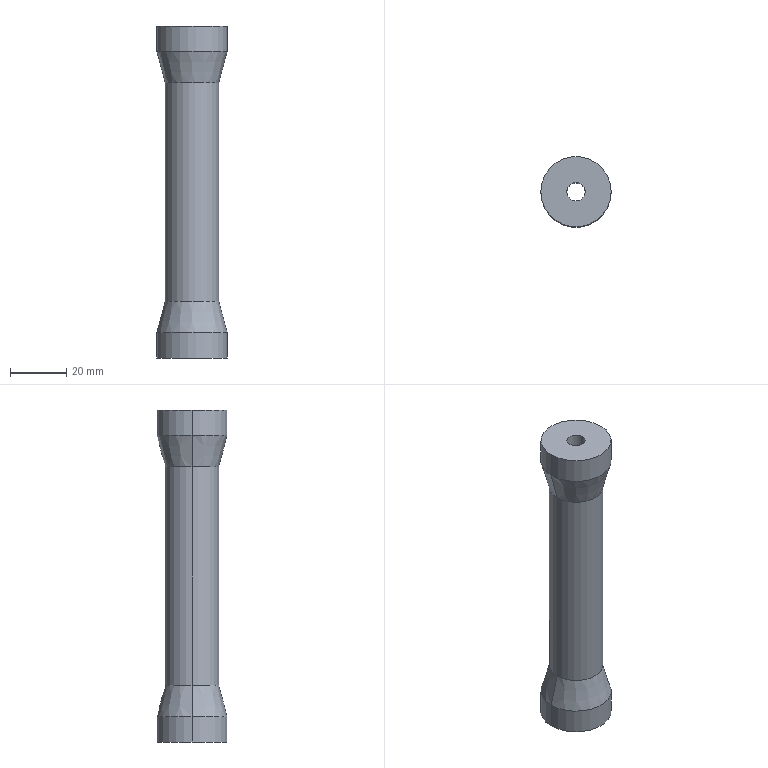Part | SolidWorks | features Extrusion 1, RevCut 1 | 1 solid | 14 faces | box 25 x 25 x 118 mm | volume 35489 mm3 | cylinder 8 | cone 4 | plane 2 | commonest cylinder face diameters 25 x4 6.5 x2 19 x2
STEP:
#1=CARTESIAN_POINT('',(9.5,0.,-38.804));
#2=VERTEX_POINT('',#1);
#3=CARTESIAN_POINT('',(-9.5,0.,-38.804));
#4=VERTEX_POINT('',#3);
#5=CARTESIAN_POINT('',(0.,0.,-38.804));
#6=DIRECTION('',(0.,0.,1.));
#7=DIRECTION('',(1.,0.,0.));
#8=AXIS2_PLACEMENT_3D('',#5,#6,#7);
#9=CIRCLE('',#8,9.5);
#10=EDGE_CURVE('',#2,#4,#9,.T.);
#11=ORIENTED_EDGE('',*,*,#10,.F.);
#12=CARTESIAN_POINT('',(12.5,0.,-50.));
#13=VERTEX_POINT('',#12);
#14=CARTESIAN_POINT('',(12.5,0.,-50.));
#15=DIRECTION('',(0.2588,0.,-0.9659));
#16=VECTOR('',#15,1000.);
#17=LINE('',#14,#16);
#18=EDGE_CURVE('',#2,#13,#17,.T.);
#19=ORIENTED_EDGE('',*,*,#18,.T.);
#20=CARTESIAN_POINT('',(-12.5,0.,-50.));
#21=VERTEX_POINT('',#20);
#22=CARTESIAN_POINT('',(0.,0.,-50.));
#23=DIRECTION('',(0.,0.,1.));
#24=DIRECTION('',(1.,0.,0.));
#25=AXIS2_PLACEMENT_3D('',#22,#23,#24);
#26=CIRCLE('',#25,12.5);
#27=EDGE_CURVE('',#13,#21,#26,.T.);
#28=ORIENTED_EDGE('',*,*,#27,.T.);
#29=CARTESIAN_POINT('',(-12.5,0.,-50.));
#30=DIRECTION('',(-0.2588,0.,-0.9659));
#31=VECTOR('',#30,1000.);
#32=LINE('',#29,#31);
#33=EDGE_CURVE('',#4,#21,#32,.T.);
#34=ORIENTED_EDGE('',*,*,#33,.F.);
#35=EDGE_LOOP('',(#11,#19,#28,#34));
#36=FACE_OUTER_BOUND('',#35,.T.);
#37=CARTESIAN_POINT('',(0.,0.,-50.));
#38=DIRECTION('',(0.,0.,-1.));
#39=DIRECTION('',(-1.,0.,0.));
#40=AXIS2_PLACEMENT_3D('',#37,#38,#39);
#41=CONICAL_SURFACE('',#40,12.5,0.2618);
#42=ADVANCED_FACE('',(#36),#41,.T.);
#43=ORIENTED_EDGE('',*,*,#10,.T.);
#44=CARTESIAN_POINT('',(-9.5,0.,38.804));
#45=VERTEX_POINT('',#44);
#46=CARTESIAN_POINT('',(-9.5,0.,0.));
#47=DIRECTION('',(0.,0.,1.));
#48=VECTOR('',#47,1000.);
#49=LINE('',#46,#48);
#50=EDGE_CURVE('',#4,#45,#49,.T.);
#51=ORIENTED_EDGE('',*,*,#50,.T.);
#52=CARTESIAN_POINT('',(9.5,0.,38.804));
#53=VERTEX_POINT('',#52);
#54=CARTESIAN_POINT('',(0.,0.,38.804));
#55=DIRECTION('',(0.,0.,1.));
#56=DIRECTION('',(1.,0.,0.));
#57=AXIS2_PLACEMENT_3D('',#54,#55,#56);
#58=CIRCLE('',#57,9.5);
#59=EDGE_CURVE('',#53,#45,#58,.T.);
#60=ORIENTED_EDGE('',*,*,#59,.F.);
#61=CARTESIAN_POINT('',(9.5,0.,0.));
#62=DIRECTION('',(0.,0.,1.));
#63=VECTOR('',#62,1000.);
#64=LINE('',#61,#63);
#65=EDGE_CURVE('',#2,#53,#64,.T.);
#66=ORIENTED_EDGE('',*,*,#65,.F.);
#67=EDGE_LOOP('',(#43,#51,#60,#66));
#68=FACE_OUTER_BOUND('',#67,.T.);
#69=CARTESIAN_POINT('',(0.,0.,0.));
#70=DIRECTION('',(0.,0.,1.));
#71=DIRECTION('',(1.,0.,0.));
#72=AXIS2_PLACEMENT_3D('',#69,#70,#71);
#73=CYLINDRICAL_SURFACE('',#72,9.5);
#74=ADVANCED_FACE('',(#68),#73,.T.);
#75=ORIENTED_EDGE('',*,*,#59,.T.);
#76=CARTESIAN_POINT('',(-12.5,0.,50.));
#77=VERTEX_POINT('',#76);
#78=CARTESIAN_POINT('',(-9.5,0.,38.804));
#79=DIRECTION('',(-0.2588,0.,0.9659));
#80=VECTOR('',#79,1000.);
#81=LINE('',#78,#80);
#82=EDGE_CURVE('',#45,#77,#81,.T.);
#83=ORIENTED_EDGE('',*,*,#82,.T.);
#84=CARTESIAN_POINT('',(12.5,0.,50.));
#85=VERTEX_POINT('',#84);
#86=CARTESIAN_POINT('',(0.,0.,50.));
#87=DIRECTION('',(0.,0.,1.));
#88=DIRECTION('',(1.,0.,0.));
#89=AXIS2_PLACEMENT_3D('',#86,#87,#88);
#90=CIRCLE('',#89,12.5);
#91=EDGE_CURVE('',#85,#77,#90,.T.);
#92=ORIENTED_EDGE('',*,*,#91,.F.);
#93=CARTESIAN_POINT('',(9.5,0.,38.804));
#94=DIRECTION('',(0.2588,0.,0.9659));
#95=VECTOR('',#94,1000.);
#96=LINE('',#93,#95);
#97=EDGE_CURVE('',#53,#85,#96,.T.);
#98=ORIENTED_EDGE('',*,*,#97,.F.);
#99=EDGE_LOOP('',(#75,#83,#92,#98));
#100=FACE_OUTER_BOUND('',#99,.T.);
#101=CARTESIAN_POINT('',(0.,0.,38.804));
#102=DIRECTION('',(0.,0.,1.));
#103=DIRECTION('',(1.,0.,0.));
#104=AXIS2_PLACEMENT_3D('',#101,#102,#103);
#105=CONICAL_SURFACE('',#104,9.5,0.2618);
#106=ADVANCED_FACE('',(#100),#105,.T.);
#107=CARTESIAN_POINT('',(-3.25,0.,59.));
#108=VERTEX_POINT('',#107);
#109=CARTESIAN_POINT('',(3.25,0.,59.));
#110=VERTEX_POINT('',#109);
#111=CARTESIAN_POINT('',(0.,0.,59.));
#112=DIRECTION('',(0.,0.,1.));
#113=DIRECTION('',(1.,0.,0.));
#114=AXIS2_PLACEMENT_3D('',#111,#112,#113);
#115=CIRCLE('',#114,3.25);
#116=EDGE_CURVE('',#108,#110,#115,.T.);
#117=ORIENTED_EDGE('',*,*,#116,.T.);
#118=CARTESIAN_POINT('',(3.25,0.,-59.));
#119=VERTEX_POINT('',#118);
#120=CARTESIAN_POINT('',(3.25,0.,59.));
#121=DIRECTION('',(0.,0.,-1.));
#122=VECTOR('',#121,1000.);
#123=LINE('',#120,#122);
#124=EDGE_CURVE('',#110,#119,#123,.T.);
#125=ORIENTED_EDGE('',*,*,#124,.T.);
#126=CARTESIAN_POINT('',(-3.25,0.,-59.));
#127=VERTEX_POINT('',#126);
#128=CARTESIAN_POINT('',(0.,0.,-59.));
#129=DIRECTION('',(0.,0.,1.));
#130=DIRECTION('',(1.,0.,0.));
#131=AXIS2_PLACEMENT_3D('',#128,#129,#130);
#132=CIRCLE('',#131,3.25);
#133=EDGE_CURVE('',#127,#119,#132,.T.);
#134=ORIENTED_EDGE('',*,*,#133,.F.);
#135=CARTESIAN_POINT('',(-3.25,0.,59.));
#136=DIRECTION('',(0.,0.,-1.));
#137=VECTOR('',#136,1000.);
#138=LINE('',#135,#137);
#139=EDGE_CURVE('',#108,#127,#138,.T.);
#140=ORIENTED_EDGE('',*,*,#139,.F.);
#141=EDGE_LOOP('',(#117,#125,#134,#140));
#142=FACE_OUTER_BOUND('',#141,.T.);
#143=CARTESIAN_POINT('',(0.,0.,59.));
#144=DIRECTION('',(0.,0.,-1.));
#145=DIRECTION('',(-1.,0.,0.));
#146=AXIS2_PLACEMENT_3D('',#143,#144,#145);
#147=CYLINDRICAL_SURFACE('',#146,3.25);
#148=ADVANCED_FACE('',(#142),#147,.F.);
#149=ORIENTED_EDGE('',*,*,#27,.F.);
#150=CARTESIAN_POINT('',(12.5,0.,-59.));
#151=VERTEX_POINT('',#150);
#152=CARTESIAN_POINT('',(12.5,0.,59.));
#153=DIRECTION('',(0.,0.,-1.));
#154=VECTOR('',#153,1000.);
#155=LINE('',#152,#154);
#156=EDGE_CURVE('',#13,#151,#155,.T.);
#157=ORIENTED_EDGE('',*,*,#156,.T.);
#158=CARTESIAN_POINT('',(-12.5,0.,-59.));
#159=VERTEX_POINT('',#158);
#160=CARTESIAN_POINT('',(0.,0.,-59.));
#161=DIRECTION('',(0.,0.,1.));
#162=DIRECTION('',(1.,0.,0.));
#163=AXIS2_PLACEMENT_3D('',#160,#161,#162);
#164=CIRCLE('',#163,12.5);
#165=EDGE_CURVE('',#151,#159,#164,.T.);
#166=ORIENTED_EDGE('',*,*,#165,.T.);
#167=CARTESIAN_POINT('',(-12.5,0.,59.));
#168=DIRECTION('',(0.,0.,-1.));
#169=VECTOR('',#168,1000.);
#170=LINE('',#167,#169);
#171=EDGE_CURVE('',#21,#159,#170,.T.);
#172=ORIENTED_EDGE('',*,*,#171,.F.);
#173=EDGE_LOOP('',(#149,#157,#166,#172));
#174=FACE_OUTER_BOUND('',#173,.T.);
#175=CARTESIAN_POINT('',(0.,0.,59.));
#176=DIRECTION('',(0.,0.,-1.));
#177=DIRECTION('',(-1.,0.,0.));
#178=AXIS2_PLACEMENT_3D('',#175,#176,#177);
#179=CYLINDRICAL_SURFACE('',#178,12.5);
#180=ADVANCED_FACE('',(#174),#179,.T.);
#181=CARTESIAN_POINT('',(12.5,0.,59.));
#182=VERTEX_POINT('',#181);
#183=CARTESIAN_POINT('',(-12.5,0.,59.));
#184=VERTEX_POINT('',#183);
#185=CARTESIAN_POINT('',(0.,0.,59.));
#186=DIRECTION('',(0.,0.,1.));
#187=DIRECTION('',(1.,0.,0.));
#188=AXIS2_PLACEMENT_3D('',#185,#186,#187);
#189=CIRCLE('',#188,12.5);
#190=EDGE_CURVE('',#182,#184,#189,.T.);
#191=ORIENTED_EDGE('',*,*,#190,.F.);
#192=CARTESIAN_POINT('',(12.5,0.,59.));
#193=DIRECTION('',(0.,0.,-1.));
#194=VECTOR('',#193,1000.);
#195=LINE('',#192,#194);
#196=EDGE_CURVE('',#182,#85,#195,.T.);
#197=ORIENTED_EDGE('',*,*,#196,.T.);
#198=ORIENTED_EDGE('',*,*,#91,.T.);
#199=CARTESIAN_POINT('',(-12.5,0.,59.));
#200=DIRECTION('',(0.,0.,-1.));
#201=VECTOR('',#200,1000.);
#202=LINE('',#199,#201);
#203=EDGE_CURVE('',#184,#77,#202,.T.);
#204=ORIENTED_EDGE('',*,*,#203,.F.);
#205=EDGE_LOOP('',(#191,#197,#198,#204));
#206=FACE_OUTER_BOUND('',#205,.T.);
#207=CARTESIAN_POINT('',(0.,0.,59.));
#208=DIRECTION('',(0.,0.,-1.));
#209=DIRECTION('',(-1.,0.,0.));
#210=AXIS2_PLACEMENT_3D('',#207,#208,#209);
#211=CYLINDRICAL_SURFACE('',#210,12.5);
#212=ADVANCED_FACE('',(#206),#211,.T.);
#213=ORIENTED_EDGE('',*,*,#196,.F.);
#214=CARTESIAN_POINT('',(0.,0.,59.));
#215=DIRECTION('',(0.,0.,1.));
#216=DIRECTION('',(1.,0.,0.));
#217=AXIS2_PLACEMENT_3D('',#214,#215,#216);
#218=CIRCLE('',#217,12.5);
#219=EDGE_CURVE('',#184,#182,#218,.T.);
#220=ORIENTED_EDGE('',*,*,#219,.F.);
#221=ORIENTED_EDGE('',*,*,#203,.T.);
#222=CARTESIAN_POINT('',(0.,0.,50.));
#223=DIRECTION('',(0.,0.,1.));
#224=DIRECTION('',(1.,0.,0.));
#225=AXIS2_PLACEMENT_3D('',#222,#223,#224);
#226=CIRCLE('',#225,12.5);
#227=EDGE_CURVE('',#77,#85,#226,.T.);
#228=ORIENTED_EDGE('',*,*,#227,.T.);
#229=EDGE_LOOP('',(#213,#220,#221,#228));
#230=FACE_OUTER_BOUND('',#229,.T.);
#231=CARTESIAN_POINT('',(0.,0.,59.));
#232=DIRECTION('',(0.,0.,-1.));
#233=DIRECTION('',(-1.,0.,0.));
#234=AXIS2_PLACEMENT_3D('',#231,#232,#233);
#235=CYLINDRICAL_SURFACE('',#234,12.5);
#236=ADVANCED_FACE('',(#230),#235,.T.);
#237=ORIENTED_EDGE('',*,*,#219,.T.);
#238=ORIENTED_EDGE('',*,*,#190,.T.);
#239=EDGE_LOOP('',(#237,#238));
#240=FACE_OUTER_BOUND('',#239,.T.);
#241=ORIENTED_EDGE('',*,*,#116,.F.);
#242=CARTESIAN_POINT('',(0.,0.,59.));
#243=DIRECTION('',(0.,0.,1.));
#244=DIRECTION('',(1.,0.,0.));
#245=AXIS2_PLACEMENT_3D('',#242,#243,#244);
#246=CIRCLE('',#245,3.25);
#247=EDGE_CURVE('',#110,#108,#246,.T.);
#248=ORIENTED_EDGE('',*,*,#247,.F.);
#249=EDGE_LOOP('',(#241,#248));
#250=FACE_BOUND('',#249,.T.);
#251=CARTESIAN_POINT('',(0.,0.,59.));
#252=DIRECTION('',(0.,0.,1.));
#253=DIRECTION('',(1.,0.,0.));
#254=AXIS2_PLACEMENT_3D('',#251,#252,#253);
#255=PLANE('',#254);
#256=ADVANCED_FACE('',(#240,#250),#255,.T.);
#257=CARTESIAN_POINT('',(0.,0.,-59.));
#258=DIRECTION('',(0.,0.,1.));
#259=DIRECTION('',(1.,0.,0.));
#260=AXIS2_PLACEMENT_3D('',#257,#258,#259);
#261=CIRCLE('',#260,12.5);
#262=EDGE_CURVE('',#159,#151,#261,.T.);
#263=ORIENTED_EDGE('',*,*,#262,.F.);
#264=ORIENTED_EDGE('',*,*,#165,.F.);
#265=EDGE_LOOP('',(#263,#264));
#266=FACE_OUTER_BOUND('',#265,.T.);
#267=ORIENTED_EDGE('',*,*,#133,.T.);
#268=CARTESIAN_POINT('',(0.,0.,-59.));
#269=DIRECTION('',(0.,0.,1.));
#270=DIRECTION('',(1.,0.,0.));
#271=AXIS2_PLACEMENT_3D('',#268,#269,#270);
#272=CIRCLE('',#271,3.25);
#273=EDGE_CURVE('',#119,#127,#272,.T.);
#274=ORIENTED_EDGE('',*,*,#273,.T.);
#275=EDGE_LOOP('',(#267,#274));
#276=FACE_BOUND('',#275,.T.);
#277=CARTESIAN_POINT('',(0.,0.,-59.));
#278=DIRECTION('',(0.,0.,1.));
#279=DIRECTION('',(1.,0.,0.));
#280=AXIS2_PLACEMENT_3D('',#277,#278,#279);
#281=PLANE('',#280);
#282=ADVANCED_FACE('',(#266,#276),#281,.F.);
#283=ORIENTED_EDGE('',*,*,#156,.F.);
#284=CARTESIAN_POINT('',(0.,0.,-50.));
#285=DIRECTION('',(0.,0.,1.));
#286=DIRECTION('',(1.,0.,0.));
#287=AXIS2_PLACEMENT_3D('',#284,#285,#286);
#288=CIRCLE('',#287,12.5);
#289=EDGE_CURVE('',#21,#13,#288,.T.);
#290=ORIENTED_EDGE('',*,*,#289,.F.);
#291=ORIENTED_EDGE('',*,*,#171,.T.);
#292=ORIENTED_EDGE('',*,*,#262,.T.);
#293=EDGE_LOOP('',(#283,#290,#291,#292));
#294=FACE_OUTER_BOUND('',#293,.T.);
#295=CARTESIAN_POINT('',(0.,0.,59.));
#296=DIRECTION('',(0.,0.,-1.));
#297=DIRECTION('',(-1.,0.,0.));
#298=AXIS2_PLACEMENT_3D('',#295,#296,#297);
#299=CYLINDRICAL_SURFACE('',#298,12.5);
#300=ADVANCED_FACE('',(#294),#299,.T.);
#301=ORIENTED_EDGE('',*,*,#124,.F.);
#302=ORIENTED_EDGE('',*,*,#247,.T.);
#303=ORIENTED_EDGE('',*,*,#139,.T.);
#304=ORIENTED_EDGE('',*,*,#273,.F.);
#305=EDGE_LOOP('',(#301,#302,#303,#304));
#306=FACE_OUTER_BOUND('',#305,.T.);
#307=CARTESIAN_POINT('',(0.,0.,59.));
#308=DIRECTION('',(0.,0.,-1.));
#309=DIRECTION('',(-1.,0.,0.));
#310=AXIS2_PLACEMENT_3D('',#307,#308,#309);
#311=CYLINDRICAL_SURFACE('',#310,3.25);
#312=ADVANCED_FACE('',(#306),#311,.F.);
#313=ORIENTED_EDGE('',*,*,#82,.F.);
#314=CARTESIAN_POINT('',(0.,0.,38.804));
#315=DIRECTION('',(0.,0.,1.));
#316=DIRECTION('',(1.,0.,0.));
#317=AXIS2_PLACEMENT_3D('',#314,#315,#316);
#318=CIRCLE('',#317,9.5);
#319=EDGE_CURVE('',#45,#53,#318,.T.);
#320=ORIENTED_EDGE('',*,*,#319,.T.);
#321=ORIENTED_EDGE('',*,*,#97,.T.);
#322=ORIENTED_EDGE('',*,*,#227,.F.);
#323=EDGE_LOOP('',(#313,#320,#321,#322));
#324=FACE_OUTER_BOUND('',#323,.T.);
#325=CARTESIAN_POINT('',(0.,0.,38.804));
#326=DIRECTION('',(0.,0.,1.));
#327=DIRECTION('',(1.,0.,0.));
#328=AXIS2_PLACEMENT_3D('',#325,#326,#327);
#329=CONICAL_SURFACE('',#328,9.5,0.2618);
#330=ADVANCED_FACE('',(#324),#329,.T.);
#331=ORIENTED_EDGE('',*,*,#50,.F.);
#332=CARTESIAN_POINT('',(0.,0.,-38.804));
#333=DIRECTION('',(0.,0.,1.));
#334=DIRECTION('',(1.,0.,0.));
#335=AXIS2_PLACEMENT_3D('',#332,#333,#334);
#336=CIRCLE('',#335,9.5);
#337=EDGE_CURVE('',#4,#2,#336,.T.);
#338=ORIENTED_EDGE('',*,*,#337,.T.);
#339=ORIENTED_EDGE('',*,*,#65,.T.);
#340=ORIENTED_EDGE('',*,*,#319,.F.);
#341=EDGE_LOOP('',(#331,#338,#339,#340));
#342=FACE_OUTER_BOUND('',#341,.T.);
#343=CARTESIAN_POINT('',(0.,0.,0.));
#344=DIRECTION('',(0.,0.,1.));
#345=DIRECTION('',(1.,0.,0.));
#346=AXIS2_PLACEMENT_3D('',#343,#344,#345);
#347=CYLINDRICAL_SURFACE('',#346,9.5);
#348=ADVANCED_FACE('',(#342),#347,.T.);
#349=ORIENTED_EDGE('',*,*,#18,.F.);
#350=ORIENTED_EDGE('',*,*,#337,.F.);
#351=ORIENTED_EDGE('',*,*,#33,.T.);
#352=ORIENTED_EDGE('',*,*,#289,.T.);
#353=EDGE_LOOP('',(#349,#350,#351,#352));
#354=FACE_OUTER_BOUND('',#353,.T.);
#355=CARTESIAN_POINT('',(0.,0.,-50.));
#356=DIRECTION('',(0.,0.,-1.));
#357=DIRECTION('',(-1.,0.,0.));
#358=AXIS2_PLACEMENT_3D('',#355,#356,#357);
#359=CONICAL_SURFACE('',#358,12.5,0.2618);
#360=ADVANCED_FACE('',(#354),#359,.T.);
#361=CLOSED_SHELL('',(#42,#74,#106,#148,#180,#212,#236,#256,#282,#300,#312,#330,#348,#360));
#362=MANIFOLD_SOLID_BREP('',#361);
#363=CARTESIAN_POINT('',(0.,0.,0.));
#364=DIRECTION('',(0.,0.,1.));
#365=DIRECTION('',(1.,0.,0.));
#366=AXIS2_PLACEMENT_3D('',#363,#364,#365);
#367=(LENGTH_UNIT()NAMED_UNIT(*)SI_UNIT(.MILLI.,.METRE.));
#368=UNCERTAINTY_MEASURE_WITH_UNIT(LENGTH_MEASURE(0.00001),#367,'','');
#369=(NAMED_UNIT(*)PLANE_ANGLE_UNIT()SI_UNIT($,.RADIAN.));
#370=(NAMED_UNIT(*)SI_UNIT($,.STERADIAN.)SOLID_ANGLE_UNIT());
#371=(GEOMETRIC_REPRESENTATION_CONTEXT(3)GLOBAL_UNCERTAINTY_ASSIGNED_CONTEXT((#368))GLOBAL_UNIT_ASSIGNED_CONTEXT((#367,#369,#370))REPRESENTATION_CONTEXT('',''));
#372=ADVANCED_BREP_SHAPE_REPRESENTATION('',(#362,#366),#371);